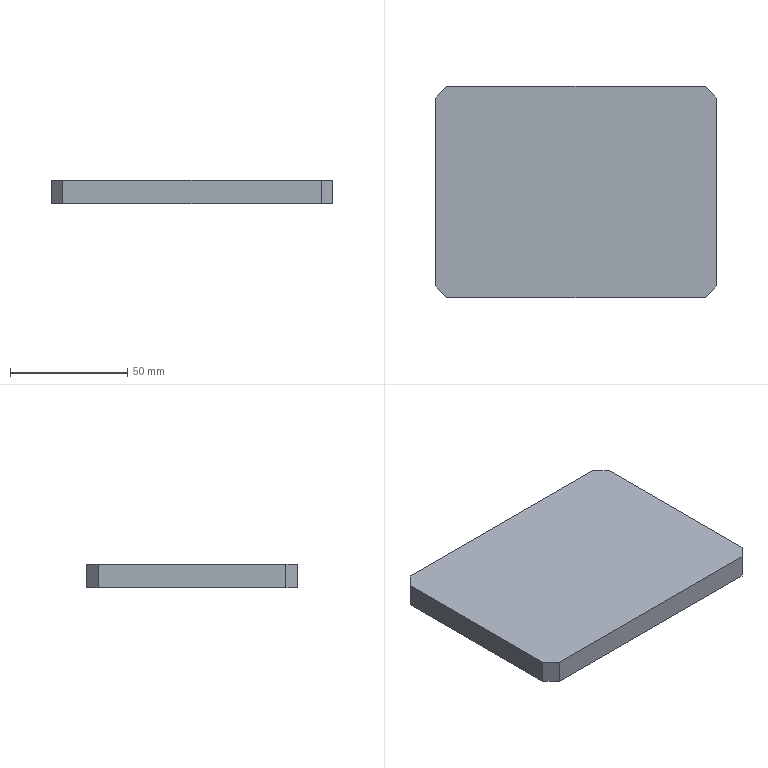Part | SolidWorks | features Chamfer 1, Extrusion 1 | 1 solid | 10 faces | box 120 x 90 x 10 mm | volume 107500 mm3 | plane 10
STEP:
#1=CARTESIAN_POINT('',(-60.,40.,0.));
#2=VERTEX_POINT('',#1);
#3=CARTESIAN_POINT('',(-60.,-40.,0.));
#4=VERTEX_POINT('',#3);
#5=CARTESIAN_POINT('',(-60.,45.,0.));
#6=DIRECTION('',(0.,-1.,0.));
#7=VECTOR('',#6,1000.);
#8=LINE('',#5,#7);
#9=EDGE_CURVE('',#2,#4,#8,.T.);
#10=ORIENTED_EDGE('',*,*,#9,.T.);
#11=CARTESIAN_POINT('',(-60.,-40.,10.));
#12=VERTEX_POINT('',#11);
#13=CARTESIAN_POINT('',(-60.,-40.,10.));
#14=DIRECTION('',(0.,0.,1.));
#15=VECTOR('',#14,1000.);
#16=LINE('',#13,#15);
#17=EDGE_CURVE('',#4,#12,#16,.T.);
#18=ORIENTED_EDGE('',*,*,#17,.T.);
#19=CARTESIAN_POINT('',(-60.,40.,10.));
#20=VERTEX_POINT('',#19);
#21=CARTESIAN_POINT('',(-60.,45.,10.));
#22=DIRECTION('',(0.,-1.,0.));
#23=VECTOR('',#22,1000.);
#24=LINE('',#21,#23);
#25=EDGE_CURVE('',#20,#12,#24,.T.);
#26=ORIENTED_EDGE('',*,*,#25,.F.);
#27=CARTESIAN_POINT('',(-60.,40.,10.));
#28=DIRECTION('',(0.,0.,-1.));
#29=VECTOR('',#28,1000.);
#30=LINE('',#27,#29);
#31=EDGE_CURVE('',#20,#2,#30,.T.);
#32=ORIENTED_EDGE('',*,*,#31,.T.);
#33=EDGE_LOOP('',(#10,#18,#26,#32));
#34=FACE_OUTER_BOUND('',#33,.T.);
#35=CARTESIAN_POINT('',(-60.,45.,10.));
#36=DIRECTION('',(1.,0.,0.));
#37=DIRECTION('',(0.,1.,0.));
#38=AXIS2_PLACEMENT_3D('',#35,#36,#37);
#39=PLANE('',#38);
#40=ADVANCED_FACE('',(#34),#39,.F.);
#41=CARTESIAN_POINT('',(-55.,-45.,0.));
#42=VERTEX_POINT('',#41);
#43=CARTESIAN_POINT('',(55.,-45.,0.));
#44=VERTEX_POINT('',#43);
#45=CARTESIAN_POINT('',(60.,-45.,0.));
#46=DIRECTION('',(1.,0.,0.));
#47=VECTOR('',#46,1000.);
#48=LINE('',#45,#47);
#49=EDGE_CURVE('',#42,#44,#48,.T.);
#50=ORIENTED_EDGE('',*,*,#49,.T.);
#51=CARTESIAN_POINT('',(55.,-45.,10.));
#52=VERTEX_POINT('',#51);
#53=CARTESIAN_POINT('',(55.,-45.,10.));
#54=DIRECTION('',(0.,0.,1.));
#55=VECTOR('',#54,1000.);
#56=LINE('',#53,#55);
#57=EDGE_CURVE('',#44,#52,#56,.T.);
#58=ORIENTED_EDGE('',*,*,#57,.T.);
#59=CARTESIAN_POINT('',(-55.,-45.,10.));
#60=VERTEX_POINT('',#59);
#61=CARTESIAN_POINT('',(60.,-45.,10.));
#62=DIRECTION('',(1.,0.,0.));
#63=VECTOR('',#62,1000.);
#64=LINE('',#61,#63);
#65=EDGE_CURVE('',#60,#52,#64,.T.);
#66=ORIENTED_EDGE('',*,*,#65,.F.);
#67=CARTESIAN_POINT('',(-55.,-45.,10.));
#68=DIRECTION('',(0.,0.,-1.));
#69=VECTOR('',#68,1000.);
#70=LINE('',#67,#69);
#71=EDGE_CURVE('',#60,#42,#70,.T.);
#72=ORIENTED_EDGE('',*,*,#71,.T.);
#73=EDGE_LOOP('',(#50,#58,#66,#72));
#74=FACE_OUTER_BOUND('',#73,.T.);
#75=CARTESIAN_POINT('',(60.,-45.,10.));
#76=DIRECTION('',(0.,1.,0.));
#77=DIRECTION('',(-1.,0.,0.));
#78=AXIS2_PLACEMENT_3D('',#75,#76,#77);
#79=PLANE('',#78);
#80=ADVANCED_FACE('',(#74),#79,.F.);
#81=CARTESIAN_POINT('',(60.,-40.,10.));
#82=VERTEX_POINT('',#81);
#83=CARTESIAN_POINT('',(60.,40.,10.));
#84=VERTEX_POINT('',#83);
#85=CARTESIAN_POINT('',(60.,45.,10.));
#86=DIRECTION('',(0.,1.,0.));
#87=VECTOR('',#86,1000.);
#88=LINE('',#85,#87);
#89=EDGE_CURVE('',#82,#84,#88,.T.);
#90=ORIENTED_EDGE('',*,*,#89,.F.);
#91=CARTESIAN_POINT('',(60.,-40.,0.));
#92=VERTEX_POINT('',#91);
#93=CARTESIAN_POINT('',(60.,-40.,10.));
#94=DIRECTION('',(0.,0.,-1.));
#95=VECTOR('',#94,1000.);
#96=LINE('',#93,#95);
#97=EDGE_CURVE('',#82,#92,#96,.T.);
#98=ORIENTED_EDGE('',*,*,#97,.T.);
#99=CARTESIAN_POINT('',(60.,40.,0.));
#100=VERTEX_POINT('',#99);
#101=CARTESIAN_POINT('',(60.,45.,0.));
#102=DIRECTION('',(0.,1.,0.));
#103=VECTOR('',#102,1000.);
#104=LINE('',#101,#103);
#105=EDGE_CURVE('',#92,#100,#104,.T.);
#106=ORIENTED_EDGE('',*,*,#105,.T.);
#107=CARTESIAN_POINT('',(60.,40.,10.));
#108=DIRECTION('',(0.,0.,1.));
#109=VECTOR('',#108,1000.);
#110=LINE('',#107,#109);
#111=EDGE_CURVE('',#100,#84,#110,.T.);
#112=ORIENTED_EDGE('',*,*,#111,.T.);
#113=EDGE_LOOP('',(#90,#98,#106,#112));
#114=FACE_OUTER_BOUND('',#113,.T.);
#115=CARTESIAN_POINT('',(60.,45.,10.));
#116=DIRECTION('',(-1.,0.,0.));
#117=DIRECTION('',(0.,-1.,0.));
#118=AXIS2_PLACEMENT_3D('',#115,#116,#117);
#119=PLANE('',#118);
#120=ADVANCED_FACE('',(#114),#119,.F.);
#121=CARTESIAN_POINT('',(55.,45.,0.));
#122=VERTEX_POINT('',#121);
#123=CARTESIAN_POINT('',(-55.,45.,0.));
#124=VERTEX_POINT('',#123);
#125=CARTESIAN_POINT('',(60.,45.,0.));
#126=DIRECTION('',(-1.,0.,0.));
#127=VECTOR('',#126,1000.);
#128=LINE('',#125,#127);
#129=EDGE_CURVE('',#122,#124,#128,.T.);
#130=ORIENTED_EDGE('',*,*,#129,.T.);
#131=CARTESIAN_POINT('',(-55.,45.,10.));
#132=VERTEX_POINT('',#131);
#133=CARTESIAN_POINT('',(-55.,45.,10.));
#134=DIRECTION('',(0.,0.,1.));
#135=VECTOR('',#134,1000.);
#136=LINE('',#133,#135);
#137=EDGE_CURVE('',#124,#132,#136,.T.);
#138=ORIENTED_EDGE('',*,*,#137,.T.);
#139=CARTESIAN_POINT('',(55.,45.,10.));
#140=VERTEX_POINT('',#139);
#141=CARTESIAN_POINT('',(60.,45.,10.));
#142=DIRECTION('',(-1.,0.,0.));
#143=VECTOR('',#142,1000.);
#144=LINE('',#141,#143);
#145=EDGE_CURVE('',#140,#132,#144,.T.);
#146=ORIENTED_EDGE('',*,*,#145,.F.);
#147=CARTESIAN_POINT('',(55.,45.,10.));
#148=DIRECTION('',(0.,0.,-1.));
#149=VECTOR('',#148,1000.);
#150=LINE('',#147,#149);
#151=EDGE_CURVE('',#140,#122,#150,.T.);
#152=ORIENTED_EDGE('',*,*,#151,.T.);
#153=EDGE_LOOP('',(#130,#138,#146,#152));
#154=FACE_OUTER_BOUND('',#153,.T.);
#155=CARTESIAN_POINT('',(60.,45.,10.));
#156=DIRECTION('',(0.,-1.,0.));
#157=DIRECTION('',(1.,0.,0.));
#158=AXIS2_PLACEMENT_3D('',#155,#156,#157);
#159=PLANE('',#158);
#160=ADVANCED_FACE('',(#154),#159,.F.);
#161=ORIENTED_EDGE('',*,*,#65,.T.);
#162=CARTESIAN_POINT('',(60.,-40.,10.));
#163=DIRECTION('',(0.7071,0.7071,0.));
#164=VECTOR('',#163,1000.);
#165=LINE('',#162,#164);
#166=EDGE_CURVE('',#52,#82,#165,.T.);
#167=ORIENTED_EDGE('',*,*,#166,.T.);
#168=ORIENTED_EDGE('',*,*,#89,.T.);
#169=CARTESIAN_POINT('',(55.,45.,10.));
#170=DIRECTION('',(-0.7071,0.7071,0.));
#171=VECTOR('',#170,1000.);
#172=LINE('',#169,#171);
#173=EDGE_CURVE('',#84,#140,#172,.T.);
#174=ORIENTED_EDGE('',*,*,#173,.T.);
#175=ORIENTED_EDGE('',*,*,#145,.T.);
#176=CARTESIAN_POINT('',(-60.,40.,10.));
#177=DIRECTION('',(-0.7071,-0.7071,0.));
#178=VECTOR('',#177,1000.);
#179=LINE('',#176,#178);
#180=EDGE_CURVE('',#132,#20,#179,.T.);
#181=ORIENTED_EDGE('',*,*,#180,.T.);
#182=ORIENTED_EDGE('',*,*,#25,.T.);
#183=CARTESIAN_POINT('',(-55.,-45.,10.));
#184=DIRECTION('',(0.7071,-0.7071,0.));
#185=VECTOR('',#184,1000.);
#186=LINE('',#183,#185);
#187=EDGE_CURVE('',#12,#60,#186,.T.);
#188=ORIENTED_EDGE('',*,*,#187,.T.);
#189=EDGE_LOOP('',(#161,#167,#168,#174,#175,#181,#182,#188));
#190=FACE_OUTER_BOUND('',#189,.T.);
#191=CARTESIAN_POINT('',(0.,0.,10.));
#192=DIRECTION('',(0.,0.,-1.));
#193=DIRECTION('',(-1.,0.,0.));
#194=AXIS2_PLACEMENT_3D('',#191,#192,#193);
#195=PLANE('',#194);
#196=ADVANCED_FACE('',(#190),#195,.F.);
#197=ORIENTED_EDGE('',*,*,#105,.F.);
#198=CARTESIAN_POINT('',(50.,-50.,0.));
#199=DIRECTION('',(-0.7071,-0.7071,0.));
#200=VECTOR('',#199,1000.);
#201=LINE('',#198,#200);
#202=EDGE_CURVE('',#92,#44,#201,.T.);
#203=ORIENTED_EDGE('',*,*,#202,.T.);
#204=ORIENTED_EDGE('',*,*,#49,.F.);
#205=CARTESIAN_POINT('',(-50.,-50.,0.));
#206=DIRECTION('',(-0.7071,0.7071,0.));
#207=VECTOR('',#206,1000.);
#208=LINE('',#205,#207);
#209=EDGE_CURVE('',#42,#4,#208,.T.);
#210=ORIENTED_EDGE('',*,*,#209,.T.);
#211=ORIENTED_EDGE('',*,*,#9,.F.);
#212=CARTESIAN_POINT('',(-50.,50.,0.));
#213=DIRECTION('',(0.7071,0.7071,0.));
#214=VECTOR('',#213,1000.);
#215=LINE('',#212,#214);
#216=EDGE_CURVE('',#2,#124,#215,.T.);
#217=ORIENTED_EDGE('',*,*,#216,.T.);
#218=ORIENTED_EDGE('',*,*,#129,.F.);
#219=CARTESIAN_POINT('',(50.,50.,0.));
#220=DIRECTION('',(0.7071,-0.7071,0.));
#221=VECTOR('',#220,1000.);
#222=LINE('',#219,#221);
#223=EDGE_CURVE('',#122,#100,#222,.T.);
#224=ORIENTED_EDGE('',*,*,#223,.T.);
#225=EDGE_LOOP('',(#197,#203,#204,#210,#211,#217,#218,#224));
#226=FACE_OUTER_BOUND('',#225,.T.);
#227=CARTESIAN_POINT('',(0.,0.,0.));
#228=DIRECTION('',(0.,0.,-1.));
#229=DIRECTION('',(-1.,0.,0.));
#230=AXIS2_PLACEMENT_3D('',#227,#228,#229);
#231=PLANE('',#230);
#232=ADVANCED_FACE('',(#226),#231,.T.);
#233=ORIENTED_EDGE('',*,*,#166,.F.);
#234=ORIENTED_EDGE('',*,*,#57,.F.);
#235=ORIENTED_EDGE('',*,*,#202,.F.);
#236=ORIENTED_EDGE('',*,*,#97,.F.);
#237=EDGE_LOOP('',(#233,#234,#235,#236));
#238=FACE_OUTER_BOUND('',#237,.T.);
#239=CARTESIAN_POINT('',(60.,-40.,10.));
#240=DIRECTION('',(-0.7071,0.7071,0.));
#241=DIRECTION('',(0.,0.,-1.));
#242=AXIS2_PLACEMENT_3D('',#239,#240,#241);
#243=PLANE('',#242);
#244=ADVANCED_FACE('',(#238),#243,.F.);
#245=ORIENTED_EDGE('',*,*,#187,.F.);
#246=ORIENTED_EDGE('',*,*,#17,.F.);
#247=ORIENTED_EDGE('',*,*,#209,.F.);
#248=ORIENTED_EDGE('',*,*,#71,.F.);
#249=EDGE_LOOP('',(#245,#246,#247,#248));
#250=FACE_OUTER_BOUND('',#249,.T.);
#251=CARTESIAN_POINT('',(-55.,-45.,10.));
#252=DIRECTION('',(0.7071,0.7071,0.));
#253=DIRECTION('',(0.,0.,-1.));
#254=AXIS2_PLACEMENT_3D('',#251,#252,#253);
#255=PLANE('',#254);
#256=ADVANCED_FACE('',(#250),#255,.F.);
#257=ORIENTED_EDGE('',*,*,#180,.F.);
#258=ORIENTED_EDGE('',*,*,#137,.F.);
#259=ORIENTED_EDGE('',*,*,#216,.F.);
#260=ORIENTED_EDGE('',*,*,#31,.F.);
#261=EDGE_LOOP('',(#257,#258,#259,#260));
#262=FACE_OUTER_BOUND('',#261,.T.);
#263=CARTESIAN_POINT('',(-60.,40.,10.));
#264=DIRECTION('',(0.7071,-0.7071,0.));
#265=DIRECTION('',(0.,0.,-1.));
#266=AXIS2_PLACEMENT_3D('',#263,#264,#265);
#267=PLANE('',#266);
#268=ADVANCED_FACE('',(#262),#267,.F.);
#269=ORIENTED_EDGE('',*,*,#173,.F.);
#270=ORIENTED_EDGE('',*,*,#111,.F.);
#271=ORIENTED_EDGE('',*,*,#223,.F.);
#272=ORIENTED_EDGE('',*,*,#151,.F.);
#273=EDGE_LOOP('',(#269,#270,#271,#272));
#274=FACE_OUTER_BOUND('',#273,.T.);
#275=CARTESIAN_POINT('',(55.,45.,10.));
#276=DIRECTION('',(-0.7071,-0.7071,0.));
#277=DIRECTION('',(0.,0.,-1.));
#278=AXIS2_PLACEMENT_3D('',#275,#276,#277);
#279=PLANE('',#278);
#280=ADVANCED_FACE('',(#274),#279,.F.);
#281=CLOSED_SHELL('',(#40,#80,#120,#160,#196,#232,#244,#256,#268,#280));
#282=MANIFOLD_SOLID_BREP('',#281);
#283=CARTESIAN_POINT('',(0.,0.,0.));
#284=DIRECTION('',(0.,0.,1.));
#285=DIRECTION('',(1.,0.,0.));
#286=AXIS2_PLACEMENT_3D('',#283,#284,#285);
#287=(LENGTH_UNIT()NAMED_UNIT(*)SI_UNIT(.MILLI.,.METRE.));
#288=UNCERTAINTY_MEASURE_WITH_UNIT(LENGTH_MEASURE(0.00001),#287,'','');
#289=(NAMED_UNIT(*)PLANE_ANGLE_UNIT()SI_UNIT($,.RADIAN.));
#290=(NAMED_UNIT(*)SI_UNIT($,.STERADIAN.)SOLID_ANGLE_UNIT());
#291=(GEOMETRIC_REPRESENTATION_CONTEXT(3)GLOBAL_UNCERTAINTY_ASSIGNED_CONTEXT((#288))GLOBAL_UNIT_ASSIGNED_CONTEXT((#287,#289,#290))REPRESENTATION_CONTEXT('',''));
#292=ADVANCED_BREP_SHAPE_REPRESENTATION('',(#282,#286),#291);